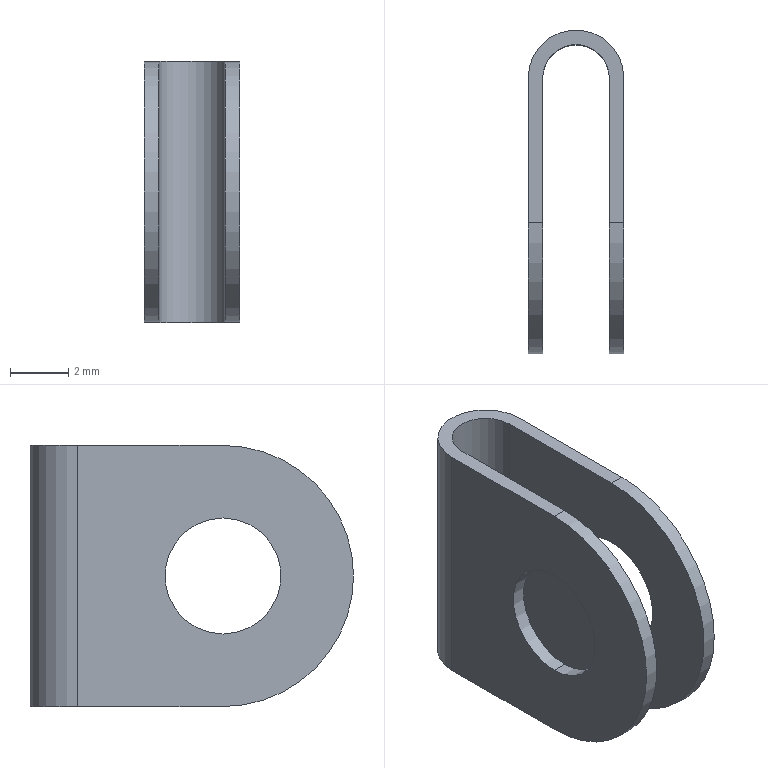Part | SolidWorks | features BaseBody 1 | 1 solid | 14 faces | box 3.3 x 11.15 x 9 mm | volume 84.034 mm3 | cylinder 8 | plane 6 | commonest cylinder face diameters 4 x4 9 x2 2.3 x1 3.3 x1
STEP:
#1=CARTESIAN_POINT('',(-60.696,1854.544,-128.5));
#2=VERTEX_POINT('',#1);
#3=CARTESIAN_POINT('',(-60.696,1854.544,-124.5));
#4=VERTEX_POINT('',#3);
#5=CARTESIAN_POINT('',(-60.696,1854.544,-126.5));
#6=DIRECTION('',(-1.,0.,0.));
#7=DIRECTION('',(0.,0.,1.));
#8=AXIS2_PLACEMENT_3D('',#5,#6,#7);
#9=CIRCLE('',#8,2.);
#10=EDGE_CURVE('',#2,#4,#9,.T.);
#11=ORIENTED_EDGE('',*,*,#10,.F.);
#12=CARTESIAN_POINT('',(-61.196,1854.544,-128.5));
#13=VERTEX_POINT('',#12);
#14=CARTESIAN_POINT('',(-60.696,1854.544,-128.5));
#15=DIRECTION('',(-1.,0.,0.));
#16=VECTOR('',#15,1000.);
#17=LINE('',#14,#16);
#18=EDGE_CURVE('',#2,#13,#17,.T.);
#19=ORIENTED_EDGE('',*,*,#18,.T.);
#20=CARTESIAN_POINT('',(-61.196,1854.544,-124.5));
#21=VERTEX_POINT('',#20);
#22=CARTESIAN_POINT('',(-61.196,1854.544,-126.5));
#23=DIRECTION('',(-1.,0.,0.));
#24=DIRECTION('',(0.,0.,1.));
#25=AXIS2_PLACEMENT_3D('',#22,#23,#24);
#26=CIRCLE('',#25,2.);
#27=EDGE_CURVE('',#13,#21,#26,.T.);
#28=ORIENTED_EDGE('',*,*,#27,.T.);
#29=CARTESIAN_POINT('',(-60.696,1854.544,-124.5));
#30=DIRECTION('',(-1.,0.,0.));
#31=VECTOR('',#30,1000.);
#32=LINE('',#29,#31);
#33=EDGE_CURVE('',#4,#21,#32,.T.);
#34=ORIENTED_EDGE('',*,*,#33,.F.);
#35=EDGE_LOOP('',(#11,#19,#28,#34));
#36=FACE_OUTER_BOUND('',#35,.T.);
#37=CARTESIAN_POINT('',(-60.696,1854.544,-126.5));
#38=DIRECTION('',(-1.,0.,0.));
#39=DIRECTION('',(0.,0.,1.));
#40=AXIS2_PLACEMENT_3D('',#37,#38,#39);
#41=CYLINDRICAL_SURFACE('',#40,2.);
#42=ADVANCED_FACE('',(#36),#41,.F.);
#43=CARTESIAN_POINT('',(-63.496,1854.544,-124.5));
#44=VERTEX_POINT('',#43);
#45=CARTESIAN_POINT('',(-63.496,1854.544,-128.5));
#46=VERTEX_POINT('',#45);
#47=CARTESIAN_POINT('',(-63.496,1854.544,-126.5));
#48=DIRECTION('',(1.,0.,0.));
#49=DIRECTION('',(0.,0.,1.));
#50=AXIS2_PLACEMENT_3D('',#47,#48,#49);
#51=CIRCLE('',#50,2.);
#52=EDGE_CURVE('',#44,#46,#51,.T.);
#53=ORIENTED_EDGE('',*,*,#52,.T.);
#54=CARTESIAN_POINT('',(-63.996,1854.544,-128.5));
#55=VERTEX_POINT('',#54);
#56=CARTESIAN_POINT('',(-60.696,1854.544,-128.5));
#57=DIRECTION('',(-1.,0.,0.));
#58=VECTOR('',#57,1000.);
#59=LINE('',#56,#58);
#60=EDGE_CURVE('',#46,#55,#59,.T.);
#61=ORIENTED_EDGE('',*,*,#60,.T.);
#62=CARTESIAN_POINT('',(-63.996,1854.544,-124.5));
#63=VERTEX_POINT('',#62);
#64=CARTESIAN_POINT('',(-63.996,1854.544,-126.5));
#65=DIRECTION('',(-1.,0.,0.));
#66=DIRECTION('',(0.,0.,1.));
#67=AXIS2_PLACEMENT_3D('',#64,#65,#66);
#68=CIRCLE('',#67,2.);
#69=EDGE_CURVE('',#55,#63,#68,.T.);
#70=ORIENTED_EDGE('',*,*,#69,.T.);
#71=CARTESIAN_POINT('',(-60.696,1854.544,-124.5));
#72=DIRECTION('',(-1.,0.,0.));
#73=VECTOR('',#72,1000.);
#74=LINE('',#71,#73);
#75=EDGE_CURVE('',#44,#63,#74,.T.);
#76=ORIENTED_EDGE('',*,*,#75,.F.);
#77=EDGE_LOOP('',(#53,#61,#70,#76));
#78=FACE_OUTER_BOUND('',#77,.T.);
#79=CARTESIAN_POINT('',(-60.696,1854.544,-126.5));
#80=DIRECTION('',(-1.,0.,0.));
#81=DIRECTION('',(0.,0.,1.));
#82=AXIS2_PLACEMENT_3D('',#79,#80,#81);
#83=CYLINDRICAL_SURFACE('',#82,2.);
#84=ADVANCED_FACE('',(#78),#83,.F.);
#85=CARTESIAN_POINT('',(-61.196,1854.544,-126.5));
#86=DIRECTION('',(-1.,0.,0.));
#87=DIRECTION('',(0.,0.,1.));
#88=AXIS2_PLACEMENT_3D('',#85,#86,#87);
#89=CIRCLE('',#88,2.);
#90=EDGE_CURVE('',#21,#13,#89,.T.);
#91=ORIENTED_EDGE('',*,*,#90,.F.);
#92=ORIENTED_EDGE('',*,*,#27,.F.);
#93=EDGE_LOOP('',(#91,#92));
#94=FACE_BOUND('',#93,.T.);
#95=CARTESIAN_POINT('',(-61.196,1859.544,-122.));
#96=VERTEX_POINT('',#95);
#97=CARTESIAN_POINT('',(-61.196,1854.544,-122.));
#98=VERTEX_POINT('',#97);
#99=CARTESIAN_POINT('',(-61.196,1859.544,-122.));
#100=DIRECTION('',(0.,-1.,0.));
#101=VECTOR('',#100,1000.);
#102=LINE('',#99,#101);
#103=EDGE_CURVE('',#96,#98,#102,.T.);
#104=ORIENTED_EDGE('',*,*,#103,.F.);
#105=CARTESIAN_POINT('',(-61.196,1859.544,-131.));
#106=VERTEX_POINT('',#105);
#107=CARTESIAN_POINT('',(-61.196,1859.544,-122.));
#108=DIRECTION('',(0.,0.,1.));
#109=VECTOR('',#108,1000.);
#110=LINE('',#107,#109);
#111=EDGE_CURVE('',#106,#96,#110,.T.);
#112=ORIENTED_EDGE('',*,*,#111,.F.);
#113=CARTESIAN_POINT('',(-61.196,1854.544,-131.));
#114=VERTEX_POINT('',#113);
#115=CARTESIAN_POINT('',(-61.196,1859.544,-131.));
#116=DIRECTION('',(0.,1.,0.));
#117=VECTOR('',#116,1000.);
#118=LINE('',#115,#117);
#119=EDGE_CURVE('',#114,#106,#118,.T.);
#120=ORIENTED_EDGE('',*,*,#119,.F.);
#121=CARTESIAN_POINT('',(-61.196,1854.544,-126.5));
#122=DIRECTION('',(1.,0.,0.));
#123=DIRECTION('',(0.,0.,-1.));
#124=AXIS2_PLACEMENT_3D('',#121,#122,#123);
#125=CIRCLE('',#124,4.5);
#126=EDGE_CURVE('',#98,#114,#125,.T.);
#127=ORIENTED_EDGE('',*,*,#126,.F.);
#128=EDGE_LOOP('',(#104,#112,#120,#127));
#129=FACE_OUTER_BOUND('',#128,.T.);
#130=CARTESIAN_POINT('',(-61.196,1859.544,-122.));
#131=DIRECTION('',(1.,0.,0.));
#132=DIRECTION('',(0.,0.,-1.));
#133=AXIS2_PLACEMENT_3D('',#130,#131,#132);
#134=PLANE('',#133);
#135=ADVANCED_FACE('',(#94,#129),#134,.F.);
#136=ORIENTED_EDGE('',*,*,#18,.F.);
#137=CARTESIAN_POINT('',(-60.696,1854.544,-126.5));
#138=DIRECTION('',(-1.,0.,0.));
#139=DIRECTION('',(0.,0.,1.));
#140=AXIS2_PLACEMENT_3D('',#137,#138,#139);
#141=CIRCLE('',#140,2.);
#142=EDGE_CURVE('',#4,#2,#141,.T.);
#143=ORIENTED_EDGE('',*,*,#142,.F.);
#144=ORIENTED_EDGE('',*,*,#33,.T.);
#145=ORIENTED_EDGE('',*,*,#90,.T.);
#146=EDGE_LOOP('',(#136,#143,#144,#145));
#147=FACE_OUTER_BOUND('',#146,.T.);
#148=CARTESIAN_POINT('',(-60.696,1854.544,-126.5));
#149=DIRECTION('',(-1.,0.,0.));
#150=DIRECTION('',(0.,0.,1.));
#151=AXIS2_PLACEMENT_3D('',#148,#149,#150);
#152=CYLINDRICAL_SURFACE('',#151,2.);
#153=ADVANCED_FACE('',(#147),#152,.F.);
#154=CARTESIAN_POINT('',(-60.696,1854.544,-122.));
#155=VERTEX_POINT('',#154);
#156=CARTESIAN_POINT('',(-62.346,1854.544,-122.));
#157=DIRECTION('',(-1.,0.,0.));
#158=VECTOR('',#157,1000.);
#159=LINE('',#156,#158);
#160=EDGE_CURVE('',#155,#98,#159,.T.);
#161=ORIENTED_EDGE('',*,*,#160,.T.);
#162=ORIENTED_EDGE('',*,*,#126,.T.);
#163=CARTESIAN_POINT('',(-60.696,1854.544,-131.));
#164=VERTEX_POINT('',#163);
#165=CARTESIAN_POINT('',(-62.346,1854.544,-131.));
#166=DIRECTION('',(1.,0.,0.));
#167=VECTOR('',#166,1000.);
#168=LINE('',#165,#167);
#169=EDGE_CURVE('',#114,#164,#168,.T.);
#170=ORIENTED_EDGE('',*,*,#169,.T.);
#171=CARTESIAN_POINT('',(-60.696,1854.544,-126.5));
#172=DIRECTION('',(-1.,0.,0.));
#173=DIRECTION('',(0.,0.,1.));
#174=AXIS2_PLACEMENT_3D('',#171,#172,#173);
#175=CIRCLE('',#174,4.5);
#176=EDGE_CURVE('',#164,#155,#175,.T.);
#177=ORIENTED_EDGE('',*,*,#176,.T.);
#178=EDGE_LOOP('',(#161,#162,#170,#177));
#179=FACE_OUTER_BOUND('',#178,.T.);
#180=CARTESIAN_POINT('',(-62.346,1854.544,-126.5));
#181=DIRECTION('',(-1.,0.,0.));
#182=DIRECTION('',(0.,0.,1.));
#183=AXIS2_PLACEMENT_3D('',#180,#181,#182);
#184=CYLINDRICAL_SURFACE('',#183,4.5);
#185=ADVANCED_FACE('',(#179),#184,.T.);
#186=CARTESIAN_POINT('',(-63.496,1859.544,-122.));
#187=VERTEX_POINT('',#186);
#188=CARTESIAN_POINT('',(-62.346,1859.544,-122.));
#189=DIRECTION('',(0.,0.,-1.));
#190=DIRECTION('',(-1.,0.,0.));
#191=AXIS2_PLACEMENT_3D('',#188,#189,#190);
#192=CIRCLE('',#191,1.15);
#193=EDGE_CURVE('',#187,#96,#192,.T.);
#194=ORIENTED_EDGE('',*,*,#193,.T.);
#195=ORIENTED_EDGE('',*,*,#103,.T.);
#196=ORIENTED_EDGE('',*,*,#160,.F.);
#197=CARTESIAN_POINT('',(-60.696,1859.544,-122.));
#198=VERTEX_POINT('',#197);
#199=CARTESIAN_POINT('',(-60.696,1859.544,-122.));
#200=DIRECTION('',(0.,1.,0.));
#201=VECTOR('',#200,1000.);
#202=LINE('',#199,#201);
#203=EDGE_CURVE('',#155,#198,#202,.T.);
#204=ORIENTED_EDGE('',*,*,#203,.T.);
#205=CARTESIAN_POINT('',(-63.996,1859.544,-122.));
#206=VERTEX_POINT('',#205);
#207=CARTESIAN_POINT('',(-62.346,1859.544,-122.));
#208=DIRECTION('',(0.,0.,1.));
#209=DIRECTION('',(-1.,0.,0.));
#210=AXIS2_PLACEMENT_3D('',#207,#208,#209);
#211=CIRCLE('',#210,1.65);
#212=EDGE_CURVE('',#198,#206,#211,.T.);
#213=ORIENTED_EDGE('',*,*,#212,.T.);
#214=CARTESIAN_POINT('',(-63.996,1854.544,-122.));
#215=VERTEX_POINT('',#214);
#216=CARTESIAN_POINT('',(-63.996,1859.544,-122.));
#217=DIRECTION('',(0.,-1.,0.));
#218=VECTOR('',#217,1000.);
#219=LINE('',#216,#218);
#220=EDGE_CURVE('',#206,#215,#219,.T.);
#221=ORIENTED_EDGE('',*,*,#220,.T.);
#222=CARTESIAN_POINT('',(-63.496,1854.544,-122.));
#223=VERTEX_POINT('',#222);
#224=CARTESIAN_POINT('',(-62.346,1854.544,-122.));
#225=DIRECTION('',(1.,0.,0.));
#226=VECTOR('',#225,1000.);
#227=LINE('',#224,#226);
#228=EDGE_CURVE('',#215,#223,#227,.T.);
#229=ORIENTED_EDGE('',*,*,#228,.T.);
#230=CARTESIAN_POINT('',(-63.496,1859.544,-122.));
#231=DIRECTION('',(0.,1.,0.));
#232=VECTOR('',#231,1000.);
#233=LINE('',#230,#232);
#234=EDGE_CURVE('',#223,#187,#233,.T.);
#235=ORIENTED_EDGE('',*,*,#234,.T.);
#236=EDGE_LOOP('',(#194,#195,#196,#204,#213,#221,#229,#235));
#237=FACE_OUTER_BOUND('',#236,.T.);
#238=CARTESIAN_POINT('',(-62.346,1859.544,-122.));
#239=DIRECTION('',(0.,0.,1.));
#240=DIRECTION('',(1.,0.,0.));
#241=AXIS2_PLACEMENT_3D('',#238,#239,#240);
#242=PLANE('',#241);
#243=ADVANCED_FACE('',(#237),#242,.T.);
#244=ORIENTED_EDGE('',*,*,#193,.F.);
#245=CARTESIAN_POINT('',(-63.496,1859.544,-131.));
#246=VERTEX_POINT('',#245);
#247=CARTESIAN_POINT('',(-63.496,1859.544,-122.));
#248=DIRECTION('',(0.,0.,1.));
#249=VECTOR('',#248,1000.);
#250=LINE('',#247,#249);
#251=EDGE_CURVE('',#246,#187,#250,.T.);
#252=ORIENTED_EDGE('',*,*,#251,.F.);
#253=CARTESIAN_POINT('',(-62.346,1859.544,-131.));
#254=DIRECTION('',(0.,0.,1.));
#255=DIRECTION('',(-1.,0.,0.));
#256=AXIS2_PLACEMENT_3D('',#253,#254,#255);
#257=CIRCLE('',#256,1.15);
#258=EDGE_CURVE('',#106,#246,#257,.T.);
#259=ORIENTED_EDGE('',*,*,#258,.F.);
#260=ORIENTED_EDGE('',*,*,#111,.T.);
#261=EDGE_LOOP('',(#244,#252,#259,#260));
#262=FACE_OUTER_BOUND('',#261,.T.);
#263=CARTESIAN_POINT('',(-62.346,1859.544,-122.));
#264=DIRECTION('',(0.,0.,-1.));
#265=DIRECTION('',(-1.,0.,0.));
#266=AXIS2_PLACEMENT_3D('',#263,#264,#265);
#267=CYLINDRICAL_SURFACE('',#266,1.15);
#268=ADVANCED_FACE('',(#262),#267,.F.);
#269=ORIENTED_EDGE('',*,*,#119,.T.);
#270=ORIENTED_EDGE('',*,*,#258,.T.);
#271=CARTESIAN_POINT('',(-63.496,1854.544,-131.));
#272=VERTEX_POINT('',#271);
#273=CARTESIAN_POINT('',(-63.496,1859.544,-131.));
#274=DIRECTION('',(0.,1.,0.));
#275=VECTOR('',#274,1000.);
#276=LINE('',#273,#275);
#277=EDGE_CURVE('',#272,#246,#276,.T.);
#278=ORIENTED_EDGE('',*,*,#277,.F.);
#279=CARTESIAN_POINT('',(-63.996,1854.544,-131.));
#280=VERTEX_POINT('',#279);
#281=CARTESIAN_POINT('',(-62.346,1854.544,-131.));
#282=DIRECTION('',(1.,0.,0.));
#283=VECTOR('',#282,1000.);
#284=LINE('',#281,#283);
#285=EDGE_CURVE('',#280,#272,#284,.T.);
#286=ORIENTED_EDGE('',*,*,#285,.F.);
#287=CARTESIAN_POINT('',(-63.996,1859.544,-131.));
#288=VERTEX_POINT('',#287);
#289=CARTESIAN_POINT('',(-63.996,1859.544,-131.));
#290=DIRECTION('',(0.,-1.,0.));
#291=VECTOR('',#290,1000.);
#292=LINE('',#289,#291);
#293=EDGE_CURVE('',#288,#280,#292,.T.);
#294=ORIENTED_EDGE('',*,*,#293,.F.);
#295=CARTESIAN_POINT('',(-60.696,1859.544,-131.));
#296=VERTEX_POINT('',#295);
#297=CARTESIAN_POINT('',(-62.346,1859.544,-131.));
#298=DIRECTION('',(0.,0.,1.));
#299=DIRECTION('',(-1.,0.,0.));
#300=AXIS2_PLACEMENT_3D('',#297,#298,#299);
#301=CIRCLE('',#300,1.65);
#302=EDGE_CURVE('',#296,#288,#301,.T.);
#303=ORIENTED_EDGE('',*,*,#302,.F.);
#304=CARTESIAN_POINT('',(-60.696,1859.544,-131.));
#305=DIRECTION('',(0.,1.,0.));
#306=VECTOR('',#305,1000.);
#307=LINE('',#304,#306);
#308=EDGE_CURVE('',#164,#296,#307,.T.);
#309=ORIENTED_EDGE('',*,*,#308,.F.);
#310=ORIENTED_EDGE('',*,*,#169,.F.);
#311=EDGE_LOOP('',(#269,#270,#278,#286,#294,#303,#309,#310));
#312=FACE_OUTER_BOUND('',#311,.T.);
#313=CARTESIAN_POINT('',(-62.346,1859.544,-131.));
#314=DIRECTION('',(0.,0.,1.));
#315=DIRECTION('',(1.,0.,0.));
#316=AXIS2_PLACEMENT_3D('',#313,#314,#315);
#317=PLANE('',#316);
#318=ADVANCED_FACE('',(#312),#317,.F.);
#319=ORIENTED_EDGE('',*,*,#142,.T.);
#320=ORIENTED_EDGE('',*,*,#10,.T.);
#321=EDGE_LOOP('',(#319,#320));
#322=FACE_BOUND('',#321,.T.);
#323=ORIENTED_EDGE('',*,*,#176,.F.);
#324=ORIENTED_EDGE('',*,*,#308,.T.);
#325=CARTESIAN_POINT('',(-60.696,1859.544,-122.));
#326=DIRECTION('',(0.,0.,-1.));
#327=VECTOR('',#326,1000.);
#328=LINE('',#325,#327);
#329=EDGE_CURVE('',#198,#296,#328,.T.);
#330=ORIENTED_EDGE('',*,*,#329,.F.);
#331=ORIENTED_EDGE('',*,*,#203,.F.);
#332=EDGE_LOOP('',(#323,#324,#330,#331));
#333=FACE_OUTER_BOUND('',#332,.T.);
#334=CARTESIAN_POINT('',(-60.696,1859.544,-122.));
#335=DIRECTION('',(-1.,0.,0.));
#336=DIRECTION('',(0.,0.,1.));
#337=AXIS2_PLACEMENT_3D('',#334,#335,#336);
#338=PLANE('',#337);
#339=ADVANCED_FACE('',(#322,#333),#338,.F.);
#340=ORIENTED_EDGE('',*,*,#52,.F.);
#341=CARTESIAN_POINT('',(-63.496,1854.544,-126.5));
#342=DIRECTION('',(1.,0.,0.));
#343=DIRECTION('',(0.,0.,1.));
#344=AXIS2_PLACEMENT_3D('',#341,#342,#343);
#345=CIRCLE('',#344,2.);
#346=EDGE_CURVE('',#46,#44,#345,.T.);
#347=ORIENTED_EDGE('',*,*,#346,.F.);
#348=EDGE_LOOP('',(#340,#347));
#349=FACE_BOUND('',#348,.T.);
#350=CARTESIAN_POINT('',(-63.496,1854.544,-126.5));
#351=DIRECTION('',(-1.,0.,0.));
#352=DIRECTION('',(0.,0.,1.));
#353=AXIS2_PLACEMENT_3D('',#350,#351,#352);
#354=CIRCLE('',#353,4.5);
#355=EDGE_CURVE('',#272,#223,#354,.T.);
#356=ORIENTED_EDGE('',*,*,#355,.F.);
#357=ORIENTED_EDGE('',*,*,#277,.T.);
#358=ORIENTED_EDGE('',*,*,#251,.T.);
#359=ORIENTED_EDGE('',*,*,#234,.F.);
#360=EDGE_LOOP('',(#356,#357,#358,#359));
#361=FACE_OUTER_BOUND('',#360,.T.);
#362=CARTESIAN_POINT('',(-63.496,1859.544,-122.));
#363=DIRECTION('',(-1.,0.,0.));
#364=DIRECTION('',(0.,0.,1.));
#365=AXIS2_PLACEMENT_3D('',#362,#363,#364);
#366=PLANE('',#365);
#367=ADVANCED_FACE('',(#349,#361),#366,.F.);
#368=ORIENTED_EDGE('',*,*,#228,.F.);
#369=CARTESIAN_POINT('',(-63.996,1854.544,-126.5));
#370=DIRECTION('',(1.,0.,0.));
#371=DIRECTION('',(0.,0.,1.));
#372=AXIS2_PLACEMENT_3D('',#369,#370,#371);
#373=CIRCLE('',#372,4.5);
#374=EDGE_CURVE('',#215,#280,#373,.T.);
#375=ORIENTED_EDGE('',*,*,#374,.T.);
#376=ORIENTED_EDGE('',*,*,#285,.T.);
#377=ORIENTED_EDGE('',*,*,#355,.T.);
#378=EDGE_LOOP('',(#368,#375,#376,#377));
#379=FACE_OUTER_BOUND('',#378,.T.);
#380=CARTESIAN_POINT('',(-62.346,1854.544,-126.5));
#381=DIRECTION('',(-1.,0.,0.));
#382=DIRECTION('',(0.,0.,1.));
#383=AXIS2_PLACEMENT_3D('',#380,#381,#382);
#384=CYLINDRICAL_SURFACE('',#383,4.5);
#385=ADVANCED_FACE('',(#379),#384,.T.);
#386=CARTESIAN_POINT('',(-63.996,1854.544,-126.5));
#387=DIRECTION('',(-1.,0.,0.));
#388=DIRECTION('',(0.,0.,1.));
#389=AXIS2_PLACEMENT_3D('',#386,#387,#388);
#390=CIRCLE('',#389,2.);
#391=EDGE_CURVE('',#63,#55,#390,.T.);
#392=ORIENTED_EDGE('',*,*,#391,.F.);
#393=ORIENTED_EDGE('',*,*,#69,.F.);
#394=EDGE_LOOP('',(#392,#393));
#395=FACE_BOUND('',#394,.T.);
#396=ORIENTED_EDGE('',*,*,#220,.F.);
#397=CARTESIAN_POINT('',(-63.996,1859.544,-122.));
#398=DIRECTION('',(0.,0.,1.));
#399=VECTOR('',#398,1000.);
#400=LINE('',#397,#399);
#401=EDGE_CURVE('',#288,#206,#400,.T.);
#402=ORIENTED_EDGE('',*,*,#401,.F.);
#403=ORIENTED_EDGE('',*,*,#293,.T.);
#404=ORIENTED_EDGE('',*,*,#374,.F.);
#405=EDGE_LOOP('',(#396,#402,#403,#404));
#406=FACE_OUTER_BOUND('',#405,.T.);
#407=CARTESIAN_POINT('',(-63.996,1859.544,-122.));
#408=DIRECTION('',(1.,0.,0.));
#409=DIRECTION('',(0.,0.,-1.));
#410=AXIS2_PLACEMENT_3D('',#407,#408,#409);
#411=PLANE('',#410);
#412=ADVANCED_FACE('',(#395,#406),#411,.F.);
#413=ORIENTED_EDGE('',*,*,#329,.T.);
#414=ORIENTED_EDGE('',*,*,#302,.T.);
#415=ORIENTED_EDGE('',*,*,#401,.T.);
#416=ORIENTED_EDGE('',*,*,#212,.F.);
#417=EDGE_LOOP('',(#413,#414,#415,#416));
#418=FACE_OUTER_BOUND('',#417,.T.);
#419=CARTESIAN_POINT('',(-62.346,1859.544,-122.));
#420=DIRECTION('',(0.,0.,-1.));
#421=DIRECTION('',(-1.,0.,0.));
#422=AXIS2_PLACEMENT_3D('',#419,#420,#421);
#423=CYLINDRICAL_SURFACE('',#422,1.65);
#424=ADVANCED_FACE('',(#418),#423,.T.);
#425=ORIENTED_EDGE('',*,*,#60,.F.);
#426=ORIENTED_EDGE('',*,*,#346,.T.);
#427=ORIENTED_EDGE('',*,*,#75,.T.);
#428=ORIENTED_EDGE('',*,*,#391,.T.);
#429=EDGE_LOOP('',(#425,#426,#427,#428));
#430=FACE_OUTER_BOUND('',#429,.T.);
#431=CARTESIAN_POINT('',(-60.696,1854.544,-126.5));
#432=DIRECTION('',(-1.,0.,0.));
#433=DIRECTION('',(0.,0.,1.));
#434=AXIS2_PLACEMENT_3D('',#431,#432,#433);
#435=CYLINDRICAL_SURFACE('',#434,2.);
#436=ADVANCED_FACE('',(#430),#435,.F.);
#437=CLOSED_SHELL('',(#42,#84,#135,#153,#185,#243,#268,#318,#339,#367,#385,#412,#424,#436));
#438=MANIFOLD_SOLID_BREP('',#437);
#439=CARTESIAN_POINT('',(0.,0.,0.));
#440=DIRECTION('',(0.,0.,1.));
#441=DIRECTION('',(1.,0.,0.));
#442=AXIS2_PLACEMENT_3D('',#439,#440,#441);
#443=(LENGTH_UNIT()NAMED_UNIT(*)SI_UNIT(.MILLI.,.METRE.));
#444=UNCERTAINTY_MEASURE_WITH_UNIT(LENGTH_MEASURE(0.00001),#443,'','');
#445=(NAMED_UNIT(*)PLANE_ANGLE_UNIT()SI_UNIT($,.RADIAN.));
#446=(NAMED_UNIT(*)SI_UNIT($,.STERADIAN.)SOLID_ANGLE_UNIT());
#447=(GEOMETRIC_REPRESENTATION_CONTEXT(3)GLOBAL_UNCERTAINTY_ASSIGNED_CONTEXT((#444))GLOBAL_UNIT_ASSIGNED_CONTEXT((#443,#445,#446))REPRESENTATION_CONTEXT('',''));
#448=ADVANCED_BREP_SHAPE_REPRESENTATION('',(#438,#442),#447);